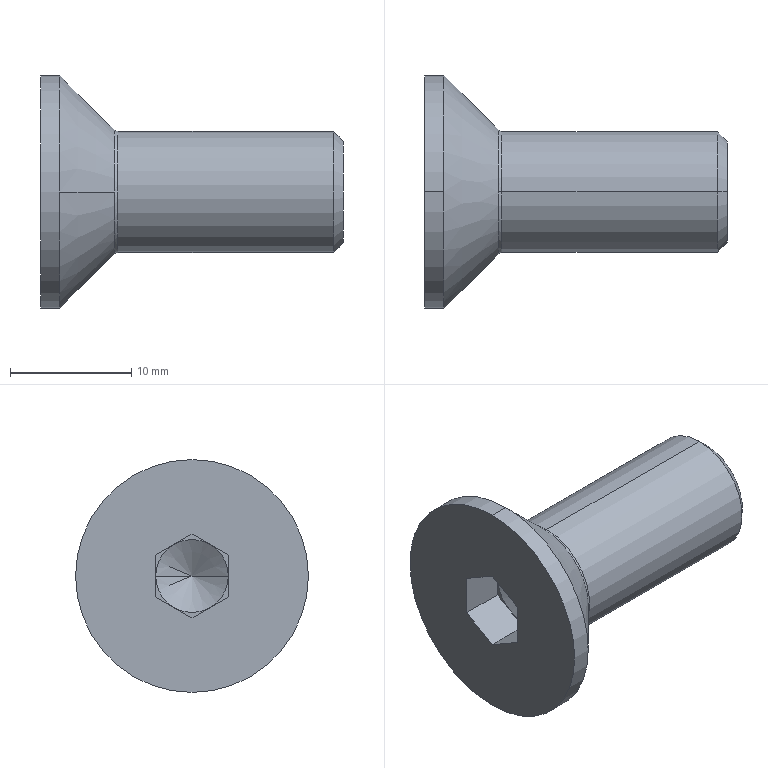Part | STEP file | hexagon socket countersunk head screws_gb_GB_FASTENER_SCREWS_HSCHS M10X25-N | 1 solid | 26 faces | box 25 x 19.22 x 19.22 mm | volume 2598 mm3 | plane 14 | cone 6 | cylinder 4 | spline 2 | commonest cylinder face diameters 10 x2 19.22 x2